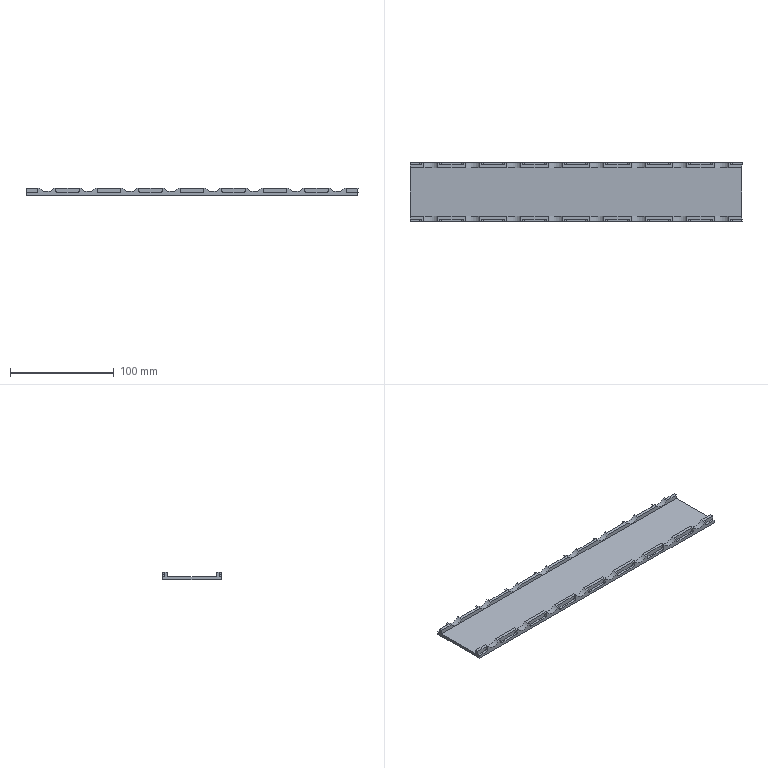NC program | Mastercam | posted with a generic post
Lines 3884 to 4970 of 9376:
(4 RC |TOOL - 3|DIA. OFF. - 3|LEN. - 3|TOOL DIA. - 4.)
N7834 T3 M6
N7836 G0 G54 G90 X11. Y-150.6 C180. B-90. S6500 M3
N7838 G43 H3 Z78.3
N7840 Z32.3
N7842 G1 Z31. F2000.
N7844 G41 D3 X7. F600.
N7846 X5.1
N7848 Y-160.
N7850 G40 Y-164.
N7852 Z30.7 F2000.
N7854 G42 D3 Y-160. F600.
N7856 Y-150.6
N7858 X7.
N7860 G40 X11.
N7862 Z30.4 F2000.
N7864 G41 D3 X7. F600.
N7866 X5.1
N7868 Y-160.
N7870 G40 Y-164.
N7872 Z30.1 F2000.
N7874 G42 D3 Y-160. F600.
N7876 Y-150.6
N7878 X7.
N7880 G40 X11.
N7882 Z29.8 F2000.
N7884 G41 D3 X7. F600.
N7886 X5.1
N7888 Y-160.
N7890 G40 Y-164.
N7892 Z29.5 F2000.
N7894 G42 D3 Y-160. F600.
N7896 Y-150.6
N7898 X7.
N7900 G40 X11.
N7902 Z29.2 F2000.
N7904 G41 D3 X7. F600.
N7906 X5.1
N7908 Y-160.
N7910 G40 Y-164.
N7912 Z28.9 F2000.
N7914 G42 D3 Y-160. F600.
N7916 Y-150.6
N7918 X7.
N7920 G40 X11.
N7922 Z28.6 F2000.
N7924 G41 D3 X7. F600.
N7926 X5.1
N7928 Y-160.
N7930 G40 Y-164.
N7932 Z28.3 F2000.
N7934 G42 D3 Y-160. F600.
N7936 Y-150.6
N7938 X7.
N7940 G40 X11.
N7942 Z28. F2000.
N7944 G41 D3 X7. F600.
N7946 X5.1
N7948 Y-160.
N7950 G40 Y-164.
N7952 Z27.7 F2000.
N7954 G42 D3 Y-160. F600.
N7956 Y-150.6
N7958 X7.
N7960 G40 X11.
N7962 Z27.4 F2000.
N7964 G41 D3 X7. F600.
N7966 X5.1
N7968 Y-160.
N7970 G40 Y-164.
N7972 Z27.1 F2000.
N7974 G42 D3 Y-160. F600.
N7976 Y-150.6
N7978 X7.
N7980 G40 X11.
N7982 Z26.8 F2000.
N7984 G41 D3 X7. F600.
N7986 X5.1
N7988 Y-160.
N7990 G40 Y-164.
N7992 Z26.5 F2000.
N7994 G42 D3 Y-160. F600.
N7996 Y-150.6
N7998 X7.
N8000 G40 X11.
N8002 Z26.2 F2000.
N8004 G41 D3 X7. F600.
N8006 X5.1
N8008 Y-160.
N8010 G40 Y-164.
N8012 G0 Z78.3
N8014 X11. Y-110.6
N8016 Z32.3
N8018 G1 Z31. F2000.
N8020 G41 D3 X7. F600.
N8022 X5.1
N8024 Y-129.4
N8026 X7.
N8028 G40 X11.
N8030 Z30.7 F2000.
N8032 G42 D3 X7. F600.
N8034 X5.1
N8036 Y-110.6
N8038 X7.
N8040 G40 X11.
N8042 Z30.4 F2000.
N8044 G41 D3 X7. F600.
N8046 X5.1
N8048 Y-129.4
N8050 X7.
N8052 G40 X11.
N8054 Z30.1 F2000.
N8056 G42 D3 X7. F600.
N8058 X5.1
N8060 Y-110.6
N8062 X7.
N8064 G40 X11.
N8066 Z29.8 F2000.
N8068 G41 D3 X7. F600.
N8070 X5.1
N8072 Y-129.4
N8074 X7.
N8076 G40 X11.
N8078 Z29.5 F2000.
N8080 G42 D3 X7. F600.
N8082 X5.1
N8084 Y-110.6
N8086 X7.
N8088 G40 X11.
N8090 Z29.2 F2000.
N8092 G41 D3 X7. F600.
N8094 X5.1
N8096 Y-129.4
N8098 X7.
N8100 G40 X11.
N8102 Z28.9 F2000.
N8104 G42 D3 X7. F600.
N8106 X5.1
N8108 Y-110.6
N8110 X7.
N8112 G40 X11.
N8114 Z28.6 F2000.
N8116 G41 D3 X7. F600.
N8118 X5.1
N8120 Y-129.4
N8122 X7.
N8124 G40 X11.
N8126 Z28.3 F2000.
N8128 G42 D3 X7. F600.
N8130 X5.1
N8132 Y-110.6
N8134 X7.
N8136 G40 X11.
N8138 Z28. F2000.
N8140 G41 D3 X7. F600.
N8142 X5.1
N8144 Y-129.4
N8146 X7.
N8148 G40 X11.
N8150 Z27.7 F2000.
N8152 G42 D3 X7. F600.
N8154 X5.1
N8156 Y-110.6
N8158 X7.
N8160 G40 X11.
N8162 Z27.4 F2000.
N8164 G41 D3 X7. F600.
N8166 X5.1
N8168 Y-129.4
N8170 X7.
N8172 G40 X11.
N8174 Z27.1 F2000.
N8176 G42 D3 X7. F600.
N8178 X5.1
N8180 Y-110.6
N8182 X7.
N8184 G40 X11.
N8186 Z26.8 F2000.
N8188 G41 D3 X7. F600.
N8190 X5.1
N8192 Y-129.4
N8194 X7.
N8196 G40 X11.
N8198 Z26.5 F2000.
N8200 G42 D3 X7. F600.
N8202 X5.1
N8204 Y-110.6
N8206 X7.
N8208 G40 X11.
N8210 Z26.2 F2000.
N8212 G41 D3 X7. F600.
N8214 X5.1
N8216 Y-129.4
N8218 X7.
N8220 G40 X11.
N8222 G0 Z78.3
N8224 Y-70.6
N8226 Z32.3
N8228 G1 Z31. F2000.
N8230 G41 D3 X7. F600.
N8232 X5.1
N8234 Y-89.4
N8236 X7.
N8238 G40 X11.
N8240 Z30.7 F2000.
N8242 G42 D3 X7. F600.
N8244 X5.1
N8246 Y-70.6
N8248 X7.
N8250 G40 X11.
N8252 Z30.4 F2000.
N8254 G41 D3 X7. F600.
N8256 X5.1
N8258 Y-89.4
N8260 X7.
N8262 G40 X11.
N8264 Z30.1 F2000.
N8266 G42 D3 X7. F600.
N8268 X5.1
N8270 Y-70.6
N8272 X7.
N8274 G40 X11.
N8276 Z29.8 F2000.
N8278 G41 D3 X7. F600.
N8280 X5.1
N8282 Y-89.4
N8284 X7.
N8286 G40 X11.
N8288 Z29.5 F2000.
N8290 G42 D3 X7. F600.
N8292 X5.1
N8294 Y-70.6
N8296 X7.
N8298 G40 X11.
N8300 Z29.2 F2000.
N8302 G41 D3 X7. F600.
N8304 X5.1
N8306 Y-89.4
N8308 X7.
N8310 G40 X11.
N8312 Z28.9 F2000.
N8314 G42 D3 X7. F600.
N8316 X5.1
N8318 Y-70.6
N8320 X7.
N8322 G40 X11.
N8324 Z28.6 F2000.
N8326 G41 D3 X7. F600.
N8328 X5.1
N8330 Y-89.4
N8332 X7.
N8334 G40 X11.
N8336 Z28.3 F2000.
N8338 G42 D3 X7. F600.
N8340 X5.1
N8342 Y-70.6
N8344 X7.
N8346 G40 X11.
N8348 Z28. F2000.
N8350 G41 D3 X7. F600.
N8352 X5.1
N8354 Y-89.4
N8356 X7.
N8358 G40 X11.
N8360 Z27.7 F2000.
N8362 G42 D3 X7. F600.
N8364 X5.1
N8366 Y-70.6
N8368 X7.
N8370 G40 X11.
N8372 Z27.4 F2000.
N8374 G41 D3 X7. F600.
N8376 X5.1
N8378 Y-89.4
N8380 X7.
N8382 G40 X11.
N8384 Z27.1 F2000.
N8386 G42 D3 X7. F600.
N8388 X5.1
N8390 Y-70.6
N8392 X7.
N8394 G40 X11.
N8396 Z26.8 F2000.
N8398 G41 D3 X7. F600.
N8400 X5.1
N8402 Y-89.4
N8404 X7.
N8406 G40 X11.
N8408 Z26.5 F2000.
N8410 G42 D3 X7. F600.
N8412 X5.1
N8414 Y-70.6
N8416 X7.
N8418 G40 X11.
N8420 Z26.2 F2000.
N8422 G41 D3 X7. F600.
N8424 X5.1
N8426 Y-89.4
N8428 X7.
N8430 G40 X11.
N8432 G0 Z78.3
N8434 Y-30.6
N8436 Z32.3
N8438 G1 Z31. F2000.
N8440 G41 D3 X7. F600.
N8442 X5.1
N8444 Y-49.4
N8446 X7.
N8448 G40 X11.
N8450 Z30.7 F2000.
N8452 G42 D3 X7. F600.
N8454 X5.1
N8456 Y-30.6
N8458 X7.
N8460 G40 X11.
N8462 Z30.4 F2000.
N8464 G41 D3 X7. F600.
N8466 X5.1
N8468 Y-49.4
N8470 X7.
N8472 G40 X11.
N8474 Z30.1 F2000.
N8476 G42 D3 X7. F600.
N8478 X5.1
N8480 Y-30.6
N8482 X7.
N8484 G40 X11.
N8486 Z29.8 F2000.
N8488 G41 D3 X7. F600.
N8490 X5.1
N8492 Y-49.4
N8494 X7.
N8496 G40 X11.
N8498 Z29.5 F2000.
N8500 G42 D3 X7. F600.
N8502 X5.1
N8504 Y-30.6
N8506 X7.
N8508 G40 X11.
N8510 Z29.2 F2000.
N8512 G41 D3 X7. F600.
N8514 X5.1
N8516 Y-49.4
N8518 X7.
N8520 G40 X11.
N8522 Z28.9 F2000.
N8524 G42 D3 X7. F600.
N8526 X5.1
N8528 Y-30.6
N8530 X7.
N8532 G40 X11.
N8534 Z28.6 F2000.
N8536 G41 D3 X7. F600.
N8538 X5.1
N8540 Y-49.4
N8542 X7.
N8544 G40 X11.
N8546 Z28.3 F2000.
N8548 G42 D3 X7. F600.
N8550 X5.1
N8552 Y-30.6
N8554 X7.
N8556 G40 X11.
N8558 Z28. F2000.
N8560 G41 D3 X7. F600.
N8562 X5.1
N8564 Y-49.4
N8566 X7.
N8568 G40 X11.
N8570 Z27.7 F2000.
N8572 G42 D3 X7. F600.
N8574 X5.1
N8576 Y-30.6
N8578 X7.
N8580 G40 X11.
N8582 Z27.4 F2000.
N8584 G41 D3 X7. F600.
N8586 X5.1
N8588 Y-49.4
N8590 X7.
N8592 G40 X11.
N8594 Z27.1 F2000.
N8596 G42 D3 X7. F600.
N8598 X5.1
N8600 Y-30.6
N8602 X7.
N8604 G40 X11.
N8606 Z26.8 F2000.
N8608 G41 D3 X7. F600.
N8610 X5.1
N8612 Y-49.4
N8614 X7.
N8616 G40 X11.
N8618 Z26.5 F2000.
N8620 G42 D3 X7. F600.
N8622 X5.1
N8624 Y-30.6
N8626 X7.
N8628 G40 X11.
N8630 Z26.2 F2000.
N8632 G41 D3 X7. F600.
N8634 X5.1
N8636 Y-49.4
N8638 X7.
N8640 G40 X11.
N8642 G0 Z78.3
N8644 Y9.4
N8646 Z32.3
N8648 G1 Z31. F2000.
N8650 G41 D3 X7. F600.
N8652 X5.1
N8654 Y-9.4
N8656 X7.
N8658 G40 X11.
N8660 Z30.7 F2000.
N8662 G42 D3 X7. F600.
N8664 X5.1
N8666 Y9.4
N8668 X7.
N8670 G40 X11.
N8672 Z30.4 F2000.
N8674 G41 D3 X7. F600.
N8676 X5.1
N8678 Y-9.4
N8680 X7.
N8682 G40 X11.
N8684 Z30.1 F2000.
N8686 G42 D3 X7. F600.
N8688 X5.1
N8690 Y9.4
N8692 X7.
N8694 G40 X11.
N8696 Z29.8 F2000.
N8698 G41 D3 X7. F600.
N8700 X5.1
N8702 Y-9.4
N8704 X7.
N8706 G40 X11.
N8708 Z29.5 F2000.
N8710 G42 D3 X7. F600.
N8712 X5.1
N8714 Y9.4
N8716 X7.
N8718 G40 X11.
N8720 Z29.2 F2000.
N8722 G41 D3 X7. F600.
N8724 X5.1
N8726 Y-9.4
N8728 X7.
N8730 G40 X11.
N8732 Z28.9 F2000.
N8734 G42 D3 X7. F600.
N8736 X5.1
N8738 Y9.4
N8740 X7.
N8742 G40 X11.
N8744 Z28.6 F2000.
N8746 G41 D3 X7. F600.
N8748 X5.1
N8750 Y-9.4
N8752 X7.
N8754 G40 X11.
N8756 Z28.3 F2000.
N8758 G42 D3 X7. F600.
N8760 X5.1
N8762 Y9.4
N8764 X7.
N8766 G40 X11.
N8768 Z28. F2000.
N8770 G41 D3 X7. F600.
N8772 X5.1
N8774 Y-9.4
N8776 X7.
N8778 G40 X11.
N8780 Z27.7 F2000.
N8782 G42 D3 X7. F600.
N8784 X5.1
N8786 Y9.4
N8788 X7.
N8790 G40 X11.
N8792 Z27.4 F2000.
N8794 G41 D3 X7. F600.
N8796 X5.1
N8798 Y-9.4
N8800 X7.
N8802 G40 X11.
N8804 Z27.1 F2000.
N8806 G42 D3 X7. F600.
N8808 X5.1
N8810 Y9.4
N8812 X7.
N8814 G40 X11.
N8816 Z26.8 F2000.
N8818 G41 D3 X7. F600.
N8820 X5.1
N8822 Y-9.4
N8824 X7.
N8826 G40 X11.
N8828 Z26.5 F2000.
N8830 G42 D3 X7. F600.
N8832 X5.1
N8834 Y9.4
N8836 X7.
N8838 G40 X11.
N8840 Z26.2 F2000.
N8842 G41 D3 X7. F600.
N8844 X5.1
N8846 Y-9.4
N8848 X7.
N8850 G40 X11.
N8852 G0 Z78.3
N8854 Y49.4
N8856 Z32.3
N8858 G1 Z31. F2000.
N8860 G41 D3 X7. F600.
N8862 X5.1
N8864 Y30.6
N8866 X7.
N8868 G40 X11.
N8870 Z30.7 F2000.
N8872 G42 D3 X7. F600.
N8874 X5.1
N8876 Y49.4
N8878 X7.
N8880 G40 X11.
N8882 Z30.4 F2000.
N8884 G41 D3 X7. F600.
N8886 X5.1
N8888 Y30.6
N8890 X7.
N8892 G40 X11.
N8894 Z30.1 F2000.
N8896 G42 D3 X7. F600.
N8898 X5.1
N8900 Y49.4
N8902 X7.
N8904 G40 X11.
N8906 Z29.8 F2000.
N8908 G41 D3 X7. F600.
N8910 X5.1
N8912 Y30.6
N8914 X7.
N8916 G40 X11.
N8918 Z29.5 F2000.
N8920 G42 D3 X7. F600.
N8922 X5.1
N8924 Y49.4
N8926 X7.
N8928 G40 X11.
N8930 Z29.2 F2000.
N8932 G41 D3 X7. F600.
N8934 X5.1
N8936 Y30.6
N8938 X7.
N8940 G40 X11.
N8942 Z28.9 F2000.
N8944 G42 D3 X7. F600.
N8946 X5.1
N8948 Y49.4
N8950 X7.
N8952 G40 X11.
N8954 Z28.6 F2000.
N8956 G41 D3 X7. F600.
N8958 X5.1
N8960 Y30.6
N8962 X7.
N8964 G40 X11.
N8966 Z28.3 F2000.
N8968 G42 D3 X7. F600.
N8970 X5.1
N8972 Y49.4
N8974 X7.
N8976 G40 X11.
N8978 Z28. F2000.
N8980 G41 D3 X7. F600.
N8982 X5.1
N8984 Y30.6
N8986 X7.
N8988 G40 X11.
N8990 Z27.7 F2000.
N8992 G42 D3 X7. F600.
N8994 X5.1
N8996 Y49.4
N8998 X7.
N9000 G40 X11.
N9002 Z27.4 F2000.
N9004 G41 D3 X7. F600.
N9006 X5.1
N9008 Y30.6
N9010 X7.
N9012 G40 X11.
N9014 Z27.1 F2000.
N9016 G42 D3 X7. F600.
N9018 X5.1
N9020 Y49.4
N9022 X7.
N9024 G40 X11.
N9026 Z26.8 F2000.
N9028 G41 D3 X7. F600.
N9030 X5.1
N9032 Y30.6
N9034 X7.
N9036 G40 X11.
N9038 Z26.5 F2000.
N9040 G42 D3 X7. F600.
N9042 X5.1
N9044 Y49.4
N9046 X7.
N9048 G40 X11.
N9050 Z26.2 F2000.
N9052 G41 D3 X7. F600.
N9054 X5.1
N9056 Y30.6
N9058 X7.
N9060 G40 X11.
N9062 G0 Z78.3
N9064 Y89.4
N9066 Z32.3
N9068 G1 Z31. F2000.
N9070 G41 D3 X7. F600.
N9072 X5.1
N9074 Y70.6
N9076 X7.
N9078 G40 X11.
N9080 Z30.7 F2000.
N9082 G42 D3 X7. F600.
N9084 X5.1
N9086 Y89.4
N9088 X7.
N9090 G40 X11.
N9092 Z30.4 F2000.
N9094 G41 D3 X7. F600.
N9096 X5.1
N9098 Y70.6
N9100 X7.
N9102 G40 X11.
N9104 Z30.1 F2000.
N9106 G42 D3 X7. F600.
N9108 X5.1
N9110 Y89.4
N9112 X7.
N9114 G40 X11.
N9116 Z29.8 F2000.
N9118 G41 D3 X7. F600.
N9120 X5.1
N9122 Y70.6
N9124 X7.
N9126 G40 X11.
N9128 Z29.5 F2000.
N9130 G42 D3 X7. F600.
N9132 X5.1
N9134 Y89.4
N9136 X7.
N9138 G40 X11.
N9140 Z29.2 F2000.
N9142 G41 D3 X7. F600.
N9144 X5.1
N9146 Y70.6
N9148 X7.
N9150 G40 X11.
N9152 Z28.9 F2000.
N9154 G42 D3 X7. F600.
N9156 X5.1
N9158 Y89.4
N9160 X7.
N9162 G40 X11.
N9164 Z28.6 F2000.
N9166 G41 D3 X7. F600.
N9168 X5.1
N9170 Y70.6
N9172 X7.
N9174 G40 X11.
N9176 Z28.3 F2000.
N9178 G42 D3 X7. F600.
N9180 X5.1
N9182 Y89.4
N9184 X7.
N9186 G40 X11.
N9188 Z28. F2000.
N9190 G41 D3 X7. F600.
N9192 X5.1
N9194 Y70.6
N9196 X7.
N9198 G40 X11.
N9200 Z27.7 F2000.
N9202 G42 D3 X7. F600.
N9204 X5.1
N9206 Y89.4
N9208 X7.
N9210 G40 X11.
N9212 Z27.4 F2000.
N9214 G41 D3 X7. F600.
N9216 X5.1
N9218 Y70.6
N9220 X7.
N9222 G40 X11.
N9224 Z27.1 F2000.
N9226 G42 D3 X7. F600.
N9228 X5.1
N9230 Y89.4
N9232 X7.
N9234 G40 X11.
N9236 Z26.8 F2000.
N9238 G41 D3 X7. F600.
N9240 X5.1
N9242 Y70.6
N9244 X7.
N9246 G40 X11.
N9248 Z26.5 F2000.
N9250 G42 D3 X7. F600.
N9252 X5.1
N9254 Y89.4
N9256 X7.
N9258 G40 X11.
N9260 Z26.2 F2000.
N9262 G41 D3 X7. F600.
N9264 X5.1
N9266 Y70.6
N9268 X7.
N9270 G40 X11.
N9272 G0 Z78.3
N9274 Y129.4
N9276 Z32.3
N9278 G1 Z31. F2000.
N9280 G41 D3 X7. F600.
N9282 X5.1
N9284 Y110.6
N9286 X7.
N9288 G40 X11.
N9290 Z30.7 F2000.
N9292 G42 D3 X7. F600.
N9294 X5.1
N9296 Y129.4
N9298 X7.
N9300 G40 X11.
N9302 Z30.4 F2000.
N9304 G41 D3 X7. F600.
N9306 X5.1
N9308 Y110.6
N9310 X7.
N9312 G40 X11.
N9314 Z30.1 F2000.
N9316 G42 D3 X7. F600.
N9318 X5.1
N9320 Y129.4
N9322 X7.
N9324 G40 X11.
N9326 Z29.8 F2000.
N9328 G41 D3 X7. F600.
N9330 X5.1
N9332 Y110.6
N9334 X7.
N9336 G40 X11.
N9338 Z29.5 F2000.
N9340 G42 D3 X7. F600.
N9342 X5.1
N9344 Y129.4
N9346 X7.
N9348 G40 X11.
N9350 Z29.2 F2000.
N9352 G41 D3 X7. F600.
N9354 X5.1
N9356 Y110.6
N9358 X7.
N9360 G40 X11.
N9362 Z28.9 F2000.
N9364 G42 D3 X7. F600.
N9366 X5.1
N9368 Y129.4
N9370 X7.
N9372 G40 X11.
N9374 Z28.6 F2000.
N9376 G41 D3 X7. F600.
N9378 X5.1
N9380 Y110.6
N9382 X7.
N9384 G40 X11.
N9386 Z28.3 F2000.
N9388 G42 D3 X7. F600.
N9390 X5.1
N9392 Y129.4
N9394 X7.
N9396 G40 X11.
N9398 Z28. F2000.
N9400 G41 D3 X7. F600.
N9402 X5.1
N9404 Y110.6
N9406 X7.
N9408 G40 X11.
N9410 Z27.7 F2000.
N9412 G42 D3 X7. F600.
N9414 X5.1
N9416 Y129.4
N9418 X7.
N9420 G40 X11.
N9422 Z27.4 F2000.
N9424 G41 D3 X7. F600.
N9426 X5.1
N9428 Y110.6
N9430 X7.
N9432 G40 X11.
N9434 Z27.1 F2000.
N9436 G42 D3 X7. F600.
N9438 X5.1
N9440 Y129.4
N9442 X7.
N9444 G40 X11.
N9446 Z26.8 F2000.
N9448 G41 D3 X7. F600.
N9450 X5.1
N9452 Y110.6
N9454 X7.
N9456 G40 X11.
N9458 Z26.5 F2000.
N9460 G42 D3 X7. F600.
N9462 X5.1
N9464 Y129.4
N9466 X7.
N9468 G40 X11.
N9470 Z26.2 F2000.
N9472 G41 D3 X7. F600.
N9474 X5.1
N9476 Y110.6
N9478 X7.
N9480 G40 X11.
N9482 G0 Z78.3
N9484 X5.1 Y164.
N9486 Z32.3
N9488 G1 Z31. F2000.
N9490 G41 D3 Y160. F600.
N9492 Y150.6
N9494 X7.
N9496 G40 X11.
N9498 Z30.7 F2000.
N9500 G42 D3 X7. F600.
N9502 X5.1
N9504 Y160.
N9506 G40 Y164.
N9508 Z30.4 F2000.
N9510 G41 D3 Y160. F600.
N9512 Y150.6
N9514 X7.
N9516 G40 X11.
N9518 Z30.1 F2000.
N9520 G42 D3 X7. F600.
N9522 X5.1
N9524 Y160.
N9526 G40 Y164.
N9528 Z29.8 F2000.
N9530 G41 D3 Y160. F600.
N9532 Y150.6
N9534 X7.
N9536 G40 X11.
N9538 Z29.5 F2000.
N9540 G42 D3 X7. F600.
N9542 X5.1
N9544 Y160.
N9546 G40 Y164.
N9548 Z29.2 F2000.
N9550 G41 D3 Y160. F600.
N9552 Y150.6
N9554 X7.
N9556 G40 X11.
N9558 Z28.9 F2000.
N9560 G42 D3 X7. F600.
N9562 X5.1
N9564 Y160.
N9566 G40 Y164.
N9568 Z28.6 F2000.
N9570 G41 D3 Y160. F600.
N9572 Y150.6
N9574 X7.
N9576 G40 X11.
N9578 Z28.3 F2000.
N9580 G42 D3 X7. F600.
N9582 X5.1
N9584 Y160.
N9586 G40 Y164.
N9588 Z28. F2000.
N9590 G41 D3 Y160. F600.
N9592 Y150.6
N9594 X7.
N9596 G40 X11.
N9598 Z27.7 F2000.
N9600 G42 D3 X7. F600.
N9602 X5.1
N9604 Y160.
N9606 G40 Y164.
N9608 Z27.4 F2000.
N9610 G41 D3 Y160. F600.
N9612 Y150.6
N9614 X7.
N9616 G40 X11.
N9618 Z27.1 F2000.
N9620 G42 D3 X7. F600.
N9622 X5.1
N9624 Y160.
N9626 G40 Y164.
N9628 Z26.8 F2000.
N9630 G41 D3 Y160. F600.
N9632 Y150.6
N9634 X7.
N9636 G40 X11.
N9638 Z26.5 F2000.
N9640 G42 D3 X7. F600.
N9642 X5.1
N9644 Y160.
N9646 G40 Y164.
N9648 Z26.2 F2000.
N9650 G41 D3 Y160. F600.
N9652 Y150.6
N9654 X7.
N9656 G40 X11.
N9658 G0 Z78.3
N9660 M5
N9662 G0 G28 G91 Z0.
N9664 G28 C0. B0.
N9666 M01
N9668 G0 G17 G40 G80 G90 G94 G98
N9670 G0 G28 G91 Z0.
(4 FI |TOOL - 4|DIA. OFF. - 4|LEN. - 4|TOOL DIA. - 4.)
N9672 T4 M6
N9674 G0 G54 G90 X11. Y-151.5 C180. B-90. S6500 M3
N9676 G43 H4 Z78.3
N9678 Z32.3
N9680 G1 Z26.1 F2000.
N9682 G41 D4 X7. F600.
N9684 X6.
N9686 Y-160.
N9688 G40 Y-164.
N9690 G0 Z78.3
N9692 X11. Y-150.5
N9694 Z32.3
N9696 G1 Z26.1 F2000.
N9698 G41 D4 X7. F600.
N9700 X5.
N9702 Y-160.
N9704 G40 Y-164.
N9706 G0 Z78.3
N9708 X11. Y-111.5
N9710 Z32.3
N9712 G1 Z26.1 F2000.
N9714 G41 D4 X7. F600.
N9716 X6.
N9718 Y-128.5
N9720 X7.
N9722 G40 X11.
N9724 G0 Z78.3
N9726 Y-110.5
N9728 Z32.3
N9730 G1 Z26.1 F2000.
N9732 G41 D4 X7. F600.
N9734 X5.
N9736 Y-129.5
N9738 X7.
N9740 G40 X11.
N9742 G0 Z78.3
N9744 Y-71.5
N9746 Z32.3
N9748 G1 Z26.1 F2000.
N9750 G41 D4 X7. F600.
N9752 X6.
N9754 Y-88.5
N9756 X7.
N9758 G40 X11.
N9760 G0 Z78.3
N9762 Y-70.5
N9764 Z32.3
N9766 G1 Z26.1 F2000.
N9768 G41 D4 X7. F600.
N9770 X5.
N9772 Y-89.5
N9774 X7.
N9776 G40 X11.
N9778 G0 Z78.3
N9780 Y-31.5
N9782 Z32.3
N9784 G1 Z26.1 F2000.
N9786 G41 D4 X7. F600.
N9788 X6.
N9790 Y-48.5
N9792 X7.
N9794 G40 X11.
N9796 G0 Z78.3
N9798 Y-30.5
N9800 Z32.3
N9802 G1 Z26.1 F2000.
N9804 G41 D4 X7. F600.
N9806 X5.
N9808 Y-49.5
N9810 X7.
N9812 G40 X11.
N9814 G0 Z78.3
N9816 Y8.5
N9818 Z32.3
N9820 G1 Z26.1 F2000.
N9822 G41 D4 X7. F600.
N9824 X6.
N9826 Y-8.5
N9828 X7.
N9830 G40 X11.
N9832 G0 Z78.3
N9834 Y9.5
N9836 Z32.3
N9838 G1 Z26.1 F2000.
N9840 G41 D4 X7. F600.
N9842 X5.
N9844 Y-9.5
N9846 X7.
N9848 G40 X11.
N9850 G0 Z78.3
N9852 Y48.5
N9854 Z32.3
N9856 G1 Z26.1 F2000.
N9858 G41 D4 X7. F600.
N9860 X6.
N9862 Y31.5
N9864 X7.
N9866 G40 X11.
N9868 G0 Z78.3
N9870 Y49.5
N9872 Z32.3
N9874 G1 Z26.1 F2000.
N9876 G41 D4 X7. F600.
N9878 X5.
N9880 Y30.5
N9882 X7.
N9884 G40 X11.
N9886 G0 Z78.3
N9888 Y88.5
N9890 Z32.3
N9892 G1 Z26.1 F2000.
N9894 G41 D4 X7. F600.
N9896 X6.
N9898 Y71.5
N9900 X7.
N9902 G40 X11.
N9904 G0 Z78.3
N9906 Y89.5
N9908 Z32.3
N9910 G1 Z26.1 F2000.
N9912 G41 D4 X7. F600.
N9914 X5.
N9916 Y70.5
N9918 X7.
N9920 G40 X11.
N9922 G0 Z78.3
N9924 Y128.5
N9926 Z32.3
N9928 G1 Z26.1 F2000.
N9930 G41 D4 X7. F600.
N9932 X6.
N9934 Y111.5
N9936 X7.
N9938 G40 X11.
N9940 G0 Z78.3
N9942 Y129.5
N9944 Z32.3
N9946 G1 Z26.1 F2000.
N9948 G41 D4 X7. F600.
N9950 X5.
N9952 Y110.5
N9954 X7.
N9956 G40 X11.
N9958 G0 Z78.3
N9960 X6. Y164.
N9962 Z32.3
N9964 G1 Z26.1 F2000.
N9966 G41 D4 Y160. F600.
N9968 Y151.5
N9970 X7.
N9972 G40 X11.
N9974 G0 Z78.3
N9976 X5. Y164.
N9978 Z32.3
N9980 G1 Z26.1 F2000.
N9982 G41 D4 Y160. F600.
N9984 Y150.5
N9986 X7.
N9988 G40 X11.
N9990 G0 Z78.3
N9992 M5
N9994 G0 G28 G91 Z0.
N9996 G28 C0. B0.
N9998 M01
N100 G0 G17 G40 G80 G90 G94 G98
N102 G0 G28 G91 Z0.